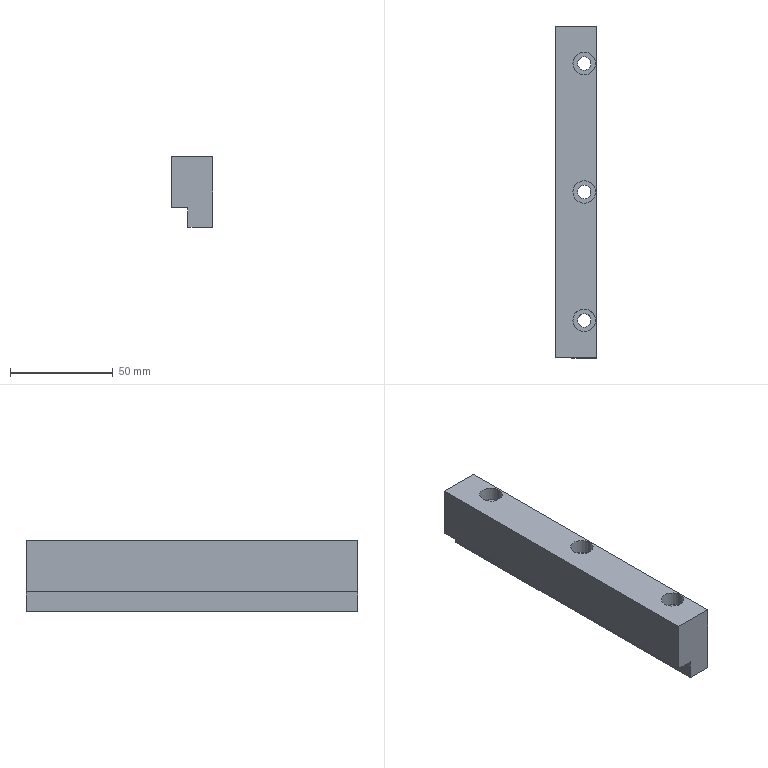Part | NX | features solid 2 | 1 solid | 17 faces | box 20 x 161.5 x 34.5 mm | volume 94428 mm3 | plane 11 | cylinder 6 | commonest cylinder face diameters 6.5 x3 11 x3
STEP:
#1=CARTESIAN_POINT('',(47.25,190.75,-35.));
#2=VERTEX_POINT('',#1);
#3=CARTESIAN_POINT('',(44.,190.75,-35.));
#4=DIRECTION('',(0.,0.,1.));
#5=DIRECTION('',(1.,0.,0.));
#6=AXIS2_PLACEMENT_3D('',#3,#4,#5);
#7=CIRCLE('',#6,3.25);
#8=EDGE_CURVE('',#2,#2,#7,.F.);
#9=ORIENTED_EDGE('',*,*,#8,.F.);
#10=EDGE_LOOP('',(#9));
#11=FACE_BOUND('',#10,.T.);
#12=CARTESIAN_POINT('',(50.,271.5,-35.));
#13=VERTEX_POINT('',#12);
#14=CARTESIAN_POINT('',(50.,110.,-35.));
#15=VERTEX_POINT('',#14);
#16=CARTESIAN_POINT('',(50.,150.,-35.));
#17=DIRECTION('',(0.,-1.,0.));
#18=VECTOR('',#17,1000.);
#19=LINE('',#16,#18);
#20=EDGE_CURVE('',#13,#15,#19,.T.);
#21=ORIENTED_EDGE('',*,*,#20,.T.);
#22=CARTESIAN_POINT('',(38.,110.,-35.));
#23=VERTEX_POINT('',#22);
#24=CARTESIAN_POINT('',(34.,110.,-35.));
#25=DIRECTION('',(-1.,0.,0.));
#26=VECTOR('',#25,1000.);
#27=LINE('',#24,#26);
#28=EDGE_CURVE('',#15,#23,#27,.T.);
#29=ORIENTED_EDGE('',*,*,#28,.T.);
#30=CARTESIAN_POINT('',(38.,271.5,-35.));
#31=VERTEX_POINT('',#30);
#32=CARTESIAN_POINT('',(38.,218.25,-35.));
#33=DIRECTION('',(0.,1.,0.));
#34=VECTOR('',#33,1000.);
#35=LINE('',#32,#34);
#36=EDGE_CURVE('',#23,#31,#35,.T.);
#37=ORIENTED_EDGE('',*,*,#36,.T.);
#38=CARTESIAN_POINT('',(0.,271.5,-35.));
#39=DIRECTION('',(-1.,0.,0.));
#40=VECTOR('',#39,1000.);
#41=LINE('',#38,#40);
#42=EDGE_CURVE('',#31,#13,#41,.F.);
#43=ORIENTED_EDGE('',*,*,#42,.T.);
#44=EDGE_LOOP('',(#21,#29,#37,#43));
#45=FACE_BOUND('',#44,.T.);
#46=CARTESIAN_POINT('',(47.25,128.25,-35.));
#47=VERTEX_POINT('',#46);
#48=CARTESIAN_POINT('',(44.,128.25,-35.));
#49=DIRECTION('',(0.,0.,1.));
#50=DIRECTION('',(1.,0.,0.));
#51=AXIS2_PLACEMENT_3D('',#48,#49,#50);
#52=CIRCLE('',#51,3.25);
#53=EDGE_CURVE('',#47,#47,#52,.F.);
#54=ORIENTED_EDGE('',*,*,#53,.F.);
#55=EDGE_LOOP('',(#54));
#56=FACE_BOUND('',#55,.T.);
#57=CARTESIAN_POINT('',(47.25,253.25,-35.));
#58=VERTEX_POINT('',#57);
#59=CARTESIAN_POINT('',(44.,253.25,-35.));
#60=DIRECTION('',(0.,0.,1.));
#61=DIRECTION('',(1.,0.,0.));
#62=AXIS2_PLACEMENT_3D('',#59,#60,#61);
#63=CIRCLE('',#62,3.25);
#64=EDGE_CURVE('',#58,#58,#63,.F.);
#65=ORIENTED_EDGE('',*,*,#64,.F.);
#66=EDGE_LOOP('',(#65));
#67=FACE_BOUND('',#66,.T.);
#68=CARTESIAN_POINT('',(0.,218.25,-35.));
#69=DIRECTION('',(0.,0.,1.));
#70=DIRECTION('',(1.,0.,0.));
#71=AXIS2_PLACEMENT_3D('',#68,#69,#70);
#72=PLANE('',#71);
#73=ADVANCED_FACE('',(#11,#45,#56,#67),#72,.F.);
#74=CARTESIAN_POINT('',(30.,271.5,-25.5));
#75=VERTEX_POINT('',#74);
#76=CARTESIAN_POINT('',(30.,271.5,-0.5));
#77=VERTEX_POINT('',#76);
#78=CARTESIAN_POINT('',(30.,271.5,-72.35));
#79=DIRECTION('',(0.,0.,-1.));
#80=VECTOR('',#79,1000.);
#81=LINE('',#78,#80);
#82=EDGE_CURVE('',#75,#77,#81,.F.);
#83=ORIENTED_EDGE('',*,*,#82,.T.);
#84=CARTESIAN_POINT('',(50.,271.5,-0.5));
#85=VERTEX_POINT('',#84);
#86=CARTESIAN_POINT('',(0.,271.5,-0.5));
#87=DIRECTION('',(-1.,0.,0.));
#88=VECTOR('',#87,1000.);
#89=LINE('',#86,#88);
#90=EDGE_CURVE('',#77,#85,#89,.F.);
#91=ORIENTED_EDGE('',*,*,#90,.T.);
#92=CARTESIAN_POINT('',(50.,271.5,-25.5));
#93=DIRECTION('',(0.,0.,-1.));
#94=VECTOR('',#93,1000.);
#95=LINE('',#92,#94);
#96=EDGE_CURVE('',#13,#85,#95,.F.);
#97=ORIENTED_EDGE('',*,*,#96,.F.);
#98=ORIENTED_EDGE('',*,*,#42,.F.);
#99=CARTESIAN_POINT('',(38.,271.5,-25.5));
#100=VERTEX_POINT('',#99);
#101=CARTESIAN_POINT('',(38.,271.5,-25.5));
#102=DIRECTION('',(0.,0.,1.));
#103=VECTOR('',#102,1000.);
#104=LINE('',#101,#103);
#105=EDGE_CURVE('',#31,#100,#104,.T.);
#106=ORIENTED_EDGE('',*,*,#105,.T.);
#107=CARTESIAN_POINT('',(0.,271.5,-25.5));
#108=DIRECTION('',(1.,0.,0.));
#109=VECTOR('',#108,1000.);
#110=LINE('',#107,#109);
#111=EDGE_CURVE('',#100,#75,#110,.F.);
#112=ORIENTED_EDGE('',*,*,#111,.T.);
#113=EDGE_LOOP('',(#83,#91,#97,#98,#106,#112));
#114=FACE_BOUND('',#113,.T.);
#115=CARTESIAN_POINT('',(0.,271.5,-72.35));
#116=DIRECTION('',(0.,-1.,0.));
#117=DIRECTION('',(0.,0.,-1.));
#118=AXIS2_PLACEMENT_3D('',#115,#116,#117);
#119=PLANE('',#118);
#120=ADVANCED_FACE('',(#114),#119,.F.);
#121=CARTESIAN_POINT('',(30.,110.,-25.5));
#122=VERTEX_POINT('',#121);
#123=CARTESIAN_POINT('',(30.,150.,-25.5));
#124=DIRECTION('',(0.,-1.,0.));
#125=VECTOR('',#124,1000.);
#126=LINE('',#123,#125);
#127=EDGE_CURVE('',#75,#122,#126,.T.);
#128=ORIENTED_EDGE('',*,*,#127,.T.);
#129=CARTESIAN_POINT('',(30.,110.,-0.5));
#130=VERTEX_POINT('',#129);
#131=CARTESIAN_POINT('',(30.,110.,-25.5));
#132=DIRECTION('',(0.,0.,1.));
#133=VECTOR('',#132,1000.);
#134=LINE('',#131,#133);
#135=EDGE_CURVE('',#122,#130,#134,.T.);
#136=ORIENTED_EDGE('',*,*,#135,.T.);
#137=CARTESIAN_POINT('',(30.,150.,-0.5));
#138=DIRECTION('',(0.,1.,0.));
#139=VECTOR('',#138,1000.);
#140=LINE('',#137,#139);
#141=EDGE_CURVE('',#130,#77,#140,.T.);
#142=ORIENTED_EDGE('',*,*,#141,.T.);
#143=ORIENTED_EDGE('',*,*,#82,.F.);
#144=EDGE_LOOP('',(#128,#136,#142,#143));
#145=FACE_BOUND('',#144,.T.);
#146=CARTESIAN_POINT('',(30.,150.,-25.5));
#147=DIRECTION('',(-1.,0.,0.));
#148=DIRECTION('',(0.,0.,1.));
#149=AXIS2_PLACEMENT_3D('',#146,#147,#148);
#150=PLANE('',#149);
#151=ADVANCED_FACE('',(#145),#150,.T.);
#152=ORIENTED_EDGE('',*,*,#36,.F.);
#153=CARTESIAN_POINT('',(38.,110.,-25.5));
#154=VERTEX_POINT('',#153);
#155=CARTESIAN_POINT('',(38.,110.,-25.5));
#156=DIRECTION('',(0.,0.,1.));
#157=VECTOR('',#156,1000.);
#158=LINE('',#155,#157);
#159=EDGE_CURVE('',#23,#154,#158,.T.);
#160=ORIENTED_EDGE('',*,*,#159,.T.);
#161=CARTESIAN_POINT('',(38.,165.,-25.5));
#162=DIRECTION('',(0.,-1.,0.));
#163=VECTOR('',#162,1000.);
#164=LINE('',#161,#163);
#165=EDGE_CURVE('',#100,#154,#164,.T.);
#166=ORIENTED_EDGE('',*,*,#165,.F.);
#167=ORIENTED_EDGE('',*,*,#105,.F.);
#168=EDGE_LOOP('',(#152,#160,#166,#167));
#169=FACE_BOUND('',#168,.T.);
#170=CARTESIAN_POINT('',(38.,165.,-25.5));
#171=DIRECTION('',(1.,0.,0.));
#172=DIRECTION('',(0.,0.,1.));
#173=AXIS2_PLACEMENT_3D('',#170,#171,#172);
#174=PLANE('',#173);
#175=ADVANCED_FACE('',(#169),#174,.F.);
#176=CARTESIAN_POINT('',(50.,110.,-0.5));
#177=VERTEX_POINT('',#176);
#178=CARTESIAN_POINT('',(50.,150.,-0.5));
#179=DIRECTION('',(0.,-1.,0.));
#180=VECTOR('',#179,1000.);
#181=LINE('',#178,#180);
#182=EDGE_CURVE('',#85,#177,#181,.T.);
#183=ORIENTED_EDGE('',*,*,#182,.T.);
#184=CARTESIAN_POINT('',(50.,110.,-25.5));
#185=DIRECTION('',(0.,0.,1.));
#186=VECTOR('',#185,1000.);
#187=LINE('',#184,#186);
#188=EDGE_CURVE('',#15,#177,#187,.T.);
#189=ORIENTED_EDGE('',*,*,#188,.F.);
#190=ORIENTED_EDGE('',*,*,#20,.F.);
#191=ORIENTED_EDGE('',*,*,#96,.T.);
#192=EDGE_LOOP('',(#183,#189,#190,#191));
#193=FACE_BOUND('',#192,.T.);
#194=CARTESIAN_POINT('',(50.,150.,-25.5));
#195=DIRECTION('',(1.,0.,0.));
#196=DIRECTION('',(0.,0.,-1.));
#197=AXIS2_PLACEMENT_3D('',#194,#195,#196);
#198=PLANE('',#197);
#199=ADVANCED_FACE('',(#193),#198,.T.);
#200=CARTESIAN_POINT('',(38.5,253.25,-0.5));
#201=VERTEX_POINT('',#200);
#202=CARTESIAN_POINT('',(44.,253.25,-0.5));
#203=DIRECTION('',(0.,0.,1.));
#204=DIRECTION('',(-1.,0.,0.));
#205=AXIS2_PLACEMENT_3D('',#202,#203,#204);
#206=CIRCLE('',#205,5.5);
#207=EDGE_CURVE('',#201,#201,#206,.T.);
#208=ORIENTED_EDGE('',*,*,#207,.F.);
#209=EDGE_LOOP('',(#208));
#210=FACE_BOUND('',#209,.T.);
#211=CARTESIAN_POINT('',(38.5,190.75,-0.5));
#212=VERTEX_POINT('',#211);
#213=CARTESIAN_POINT('',(44.,190.75,-0.5));
#214=DIRECTION('',(0.,0.,1.));
#215=DIRECTION('',(-1.,0.,0.));
#216=AXIS2_PLACEMENT_3D('',#213,#214,#215);
#217=CIRCLE('',#216,5.5);
#218=EDGE_CURVE('',#212,#212,#217,.T.);
#219=ORIENTED_EDGE('',*,*,#218,.F.);
#220=EDGE_LOOP('',(#219));
#221=FACE_BOUND('',#220,.T.);
#222=CARTESIAN_POINT('',(38.5,128.25,-0.5));
#223=VERTEX_POINT('',#222);
#224=CARTESIAN_POINT('',(44.,128.25,-0.5));
#225=DIRECTION('',(0.,0.,1.));
#226=DIRECTION('',(-1.,0.,0.));
#227=AXIS2_PLACEMENT_3D('',#224,#225,#226);
#228=CIRCLE('',#227,5.5);
#229=EDGE_CURVE('',#223,#223,#228,.T.);
#230=ORIENTED_EDGE('',*,*,#229,.F.);
#231=EDGE_LOOP('',(#230));
#232=FACE_BOUND('',#231,.T.);
#233=ORIENTED_EDGE('',*,*,#141,.F.);
#234=CARTESIAN_POINT('',(34.,110.,-0.5));
#235=DIRECTION('',(-1.,0.,0.));
#236=VECTOR('',#235,1000.);
#237=LINE('',#234,#236);
#238=EDGE_CURVE('',#177,#130,#237,.T.);
#239=ORIENTED_EDGE('',*,*,#238,.F.);
#240=ORIENTED_EDGE('',*,*,#182,.F.);
#241=ORIENTED_EDGE('',*,*,#90,.F.);
#242=EDGE_LOOP('',(#233,#239,#240,#241));
#243=FACE_BOUND('',#242,.T.);
#244=CARTESIAN_POINT('',(11.5,150.,-0.5));
#245=DIRECTION('',(0.,0.,1.));
#246=DIRECTION('',(0.,-1.,0.));
#247=AXIS2_PLACEMENT_3D('',#244,#245,#246);
#248=PLANE('',#247);
#249=ADVANCED_FACE('',(#210,#221,#232,#243),#248,.T.);
#250=ORIENTED_EDGE('',*,*,#165,.T.);
#251=CARTESIAN_POINT('',(34.,110.,-25.5));
#252=DIRECTION('',(1.,0.,0.));
#253=VECTOR('',#252,1000.);
#254=LINE('',#251,#253);
#255=EDGE_CURVE('',#122,#154,#254,.T.);
#256=ORIENTED_EDGE('',*,*,#255,.F.);
#257=ORIENTED_EDGE('',*,*,#127,.F.);
#258=ORIENTED_EDGE('',*,*,#111,.F.);
#259=EDGE_LOOP('',(#250,#256,#257,#258));
#260=FACE_BOUND('',#259,.T.);
#261=CARTESIAN_POINT('',(34.,150.,-25.5));
#262=DIRECTION('',(0.,0.,-1.));
#263=DIRECTION('',(-1.,0.,0.));
#264=AXIS2_PLACEMENT_3D('',#261,#262,#263);
#265=PLANE('',#264);
#266=ADVANCED_FACE('',(#260),#265,.T.);
#267=ORIENTED_EDGE('',*,*,#28,.F.);
#268=ORIENTED_EDGE('',*,*,#188,.T.);
#269=ORIENTED_EDGE('',*,*,#238,.T.);
#270=ORIENTED_EDGE('',*,*,#135,.F.);
#271=ORIENTED_EDGE('',*,*,#255,.T.);
#272=ORIENTED_EDGE('',*,*,#159,.F.);
#273=EDGE_LOOP('',(#267,#268,#269,#270,#271,#272));
#274=FACE_BOUND('',#273,.T.);
#275=CARTESIAN_POINT('',(34.,110.,-25.5));
#276=DIRECTION('',(0.,-1.,0.));
#277=DIRECTION('',(0.,0.,-1.));
#278=AXIS2_PLACEMENT_3D('',#275,#276,#277);
#279=PLANE('',#278);
#280=ADVANCED_FACE('',(#274),#279,.T.);
#281=CARTESIAN_POINT('',(47.25,128.25,-7.5));
#282=VERTEX_POINT('',#281);
#283=CARTESIAN_POINT('',(44.,128.25,-7.5));
#284=DIRECTION('',(0.,0.,1.));
#285=DIRECTION('',(1.,0.,0.));
#286=AXIS2_PLACEMENT_3D('',#283,#284,#285);
#287=CIRCLE('',#286,3.25);
#288=EDGE_CURVE('',#282,#282,#287,.F.);
#289=ORIENTED_EDGE('',*,*,#288,.T.);
#290=EDGE_LOOP('',(#289));
#291=FACE_BOUND('',#290,.T.);
#292=CARTESIAN_POINT('',(38.5,128.25,-7.5));
#293=VERTEX_POINT('',#292);
#294=CARTESIAN_POINT('',(44.,128.25,-7.5));
#295=DIRECTION('',(0.,0.,-1.));
#296=DIRECTION('',(-1.,0.,0.));
#297=AXIS2_PLACEMENT_3D('',#294,#295,#296);
#298=CIRCLE('',#297,5.5);
#299=EDGE_CURVE('',#293,#293,#298,.F.);
#300=ORIENTED_EDGE('',*,*,#299,.T.);
#301=EDGE_LOOP('',(#300));
#302=FACE_BOUND('',#301,.T.);
#303=CARTESIAN_POINT('',(44.,128.25,-7.5));
#304=DIRECTION('',(0.,0.,-1.));
#305=DIRECTION('',(1.,0.,0.));
#306=AXIS2_PLACEMENT_3D('',#303,#304,#305);
#307=PLANE('',#306);
#308=ADVANCED_FACE('',(#291,#302),#307,.F.);
#309=ORIENTED_EDGE('',*,*,#299,.F.);
#310=EDGE_LOOP('',(#309));
#311=FACE_BOUND('',#310,.T.);
#312=ORIENTED_EDGE('',*,*,#229,.T.);
#313=EDGE_LOOP('',(#312));
#314=FACE_BOUND('',#313,.T.);
#315=CARTESIAN_POINT('',(44.,128.25,-0.5));
#316=DIRECTION('',(0.,0.,-1.));
#317=DIRECTION('',(-1.,0.,0.));
#318=AXIS2_PLACEMENT_3D('',#315,#316,#317);
#319=CYLINDRICAL_SURFACE('',#318,5.5);
#320=ADVANCED_FACE('',(#311,#314),#319,.F.);
#321=ORIENTED_EDGE('',*,*,#288,.F.);
#322=EDGE_LOOP('',(#321));
#323=FACE_BOUND('',#322,.T.);
#324=ORIENTED_EDGE('',*,*,#53,.T.);
#325=EDGE_LOOP('',(#324));
#326=FACE_BOUND('',#325,.T.);
#327=CARTESIAN_POINT('',(44.,128.25,-0.5));
#328=DIRECTION('',(0.,0.,-1.));
#329=DIRECTION('',(-1.,0.,0.));
#330=AXIS2_PLACEMENT_3D('',#327,#328,#329);
#331=CYLINDRICAL_SURFACE('',#330,3.25);
#332=ADVANCED_FACE('',(#323,#326),#331,.F.);
#333=CARTESIAN_POINT('',(47.25,190.75,-7.5));
#334=VERTEX_POINT('',#333);
#335=CARTESIAN_POINT('',(44.,190.75,-7.5));
#336=DIRECTION('',(0.,0.,1.));
#337=DIRECTION('',(1.,0.,0.));
#338=AXIS2_PLACEMENT_3D('',#335,#336,#337);
#339=CIRCLE('',#338,3.25);
#340=EDGE_CURVE('',#334,#334,#339,.F.);
#341=ORIENTED_EDGE('',*,*,#340,.T.);
#342=EDGE_LOOP('',(#341));
#343=FACE_BOUND('',#342,.T.);
#344=CARTESIAN_POINT('',(38.5,190.75,-7.5));
#345=VERTEX_POINT('',#344);
#346=CARTESIAN_POINT('',(44.,190.75,-7.5));
#347=DIRECTION('',(0.,0.,-1.));
#348=DIRECTION('',(-1.,0.,0.));
#349=AXIS2_PLACEMENT_3D('',#346,#347,#348);
#350=CIRCLE('',#349,5.5);
#351=EDGE_CURVE('',#345,#345,#350,.F.);
#352=ORIENTED_EDGE('',*,*,#351,.T.);
#353=EDGE_LOOP('',(#352));
#354=FACE_BOUND('',#353,.T.);
#355=CARTESIAN_POINT('',(44.,190.75,-7.5));
#356=DIRECTION('',(0.,0.,-1.));
#357=DIRECTION('',(1.,0.,0.));
#358=AXIS2_PLACEMENT_3D('',#355,#356,#357);
#359=PLANE('',#358);
#360=ADVANCED_FACE('',(#343,#354),#359,.F.);
#361=ORIENTED_EDGE('',*,*,#351,.F.);
#362=EDGE_LOOP('',(#361));
#363=FACE_BOUND('',#362,.T.);
#364=ORIENTED_EDGE('',*,*,#218,.T.);
#365=EDGE_LOOP('',(#364));
#366=FACE_BOUND('',#365,.T.);
#367=CARTESIAN_POINT('',(44.,190.75,-0.5));
#368=DIRECTION('',(0.,0.,-1.));
#369=DIRECTION('',(-1.,0.,0.));
#370=AXIS2_PLACEMENT_3D('',#367,#368,#369);
#371=CYLINDRICAL_SURFACE('',#370,5.5);
#372=ADVANCED_FACE('',(#363,#366),#371,.F.);
#373=ORIENTED_EDGE('',*,*,#340,.F.);
#374=EDGE_LOOP('',(#373));
#375=FACE_BOUND('',#374,.T.);
#376=ORIENTED_EDGE('',*,*,#8,.T.);
#377=EDGE_LOOP('',(#376));
#378=FACE_BOUND('',#377,.T.);
#379=CARTESIAN_POINT('',(44.,190.75,-0.5));
#380=DIRECTION('',(0.,0.,-1.));
#381=DIRECTION('',(-1.,0.,0.));
#382=AXIS2_PLACEMENT_3D('',#379,#380,#381);
#383=CYLINDRICAL_SURFACE('',#382,3.25);
#384=ADVANCED_FACE('',(#375,#378),#383,.F.);
#385=CARTESIAN_POINT('',(47.25,253.25,-7.5));
#386=VERTEX_POINT('',#385);
#387=CARTESIAN_POINT('',(44.,253.25,-7.5));
#388=DIRECTION('',(0.,0.,1.));
#389=DIRECTION('',(1.,0.,0.));
#390=AXIS2_PLACEMENT_3D('',#387,#388,#389);
#391=CIRCLE('',#390,3.25);
#392=EDGE_CURVE('',#386,#386,#391,.F.);
#393=ORIENTED_EDGE('',*,*,#392,.T.);
#394=EDGE_LOOP('',(#393));
#395=FACE_BOUND('',#394,.T.);
#396=CARTESIAN_POINT('',(38.5,253.25,-7.5));
#397=VERTEX_POINT('',#396);
#398=CARTESIAN_POINT('',(44.,253.25,-7.5));
#399=DIRECTION('',(0.,0.,-1.));
#400=DIRECTION('',(-1.,0.,0.));
#401=AXIS2_PLACEMENT_3D('',#398,#399,#400);
#402=CIRCLE('',#401,5.5);
#403=EDGE_CURVE('',#397,#397,#402,.F.);
#404=ORIENTED_EDGE('',*,*,#403,.T.);
#405=EDGE_LOOP('',(#404));
#406=FACE_BOUND('',#405,.T.);
#407=CARTESIAN_POINT('',(44.,253.25,-7.5));
#408=DIRECTION('',(0.,0.,-1.));
#409=DIRECTION('',(1.,0.,0.));
#410=AXIS2_PLACEMENT_3D('',#407,#408,#409);
#411=PLANE('',#410);
#412=ADVANCED_FACE('',(#395,#406),#411,.F.);
#413=ORIENTED_EDGE('',*,*,#403,.F.);
#414=EDGE_LOOP('',(#413));
#415=FACE_BOUND('',#414,.T.);
#416=ORIENTED_EDGE('',*,*,#207,.T.);
#417=EDGE_LOOP('',(#416));
#418=FACE_BOUND('',#417,.T.);
#419=CARTESIAN_POINT('',(44.,253.25,-0.5));
#420=DIRECTION('',(0.,0.,-1.));
#421=DIRECTION('',(-1.,0.,0.));
#422=AXIS2_PLACEMENT_3D('',#419,#420,#421);
#423=CYLINDRICAL_SURFACE('',#422,5.5);
#424=ADVANCED_FACE('',(#415,#418),#423,.F.);
#425=ORIENTED_EDGE('',*,*,#392,.F.);
#426=EDGE_LOOP('',(#425));
#427=FACE_BOUND('',#426,.T.);
#428=ORIENTED_EDGE('',*,*,#64,.T.);
#429=EDGE_LOOP('',(#428));
#430=FACE_BOUND('',#429,.T.);
#431=CARTESIAN_POINT('',(44.,253.25,-0.5));
#432=DIRECTION('',(0.,0.,-1.));
#433=DIRECTION('',(-1.,0.,0.));
#434=AXIS2_PLACEMENT_3D('',#431,#432,#433);
#435=CYLINDRICAL_SURFACE('',#434,3.25);
#436=ADVANCED_FACE('',(#427,#430),#435,.F.);
#437=CLOSED_SHELL('',(#73,#120,#151,#175,#199,#249,#266,#280,#308,#320,#332,#360,#372,#384,#412,#424,#436));
#438=MANIFOLD_SOLID_BREP('',#437);
#439=(LENGTH_UNIT()NAMED_UNIT(*)SI_UNIT(.MILLI.,.METRE.));
#440=UNCERTAINTY_MEASURE_WITH_UNIT(LENGTH_MEASURE(0.00001),#439,'','');
#441=(NAMED_UNIT(*)PLANE_ANGLE_UNIT()SI_UNIT($,.RADIAN.));
#442=(NAMED_UNIT(*)SI_UNIT($,.STERADIAN.)SOLID_ANGLE_UNIT());
#443=(GEOMETRIC_REPRESENTATION_CONTEXT(3)GLOBAL_UNCERTAINTY_ASSIGNED_CONTEXT((#440))GLOBAL_UNIT_ASSIGNED_CONTEXT((#439,#441,#442))REPRESENTATION_CONTEXT('',''));
#444=ADVANCED_BREP_SHAPE_REPRESENTATION('',(#438),#443);